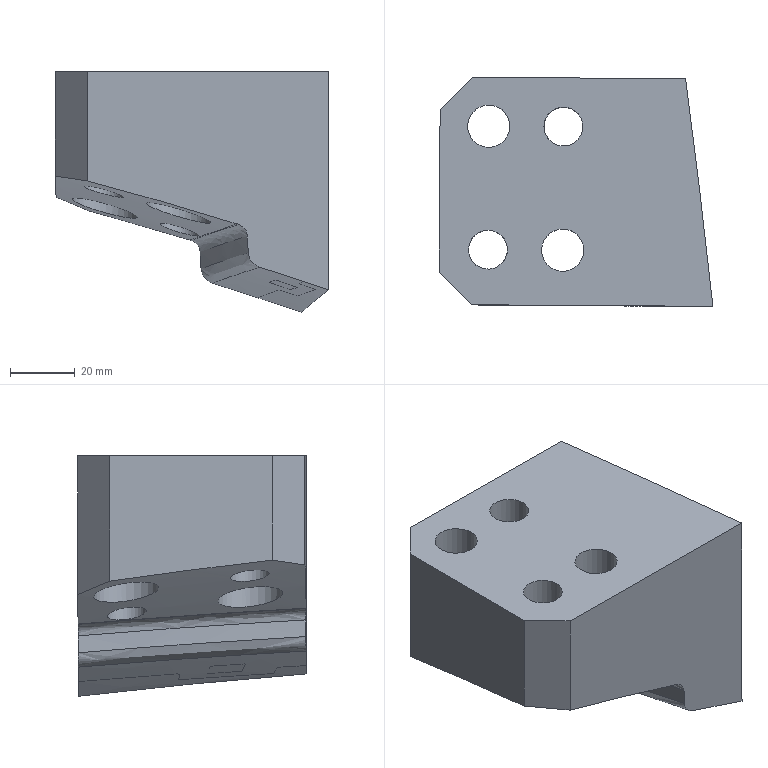Part | NX | features MAIN_BODY 2 | 1 solid | 23 faces | box 84.282 x 70.472 x 74.024 mm | volume 250188 mm3 | spline 9 | plane 8 | cylinder 6 | commonest cylinder face diameters 12 x2 13 x2 20 x2